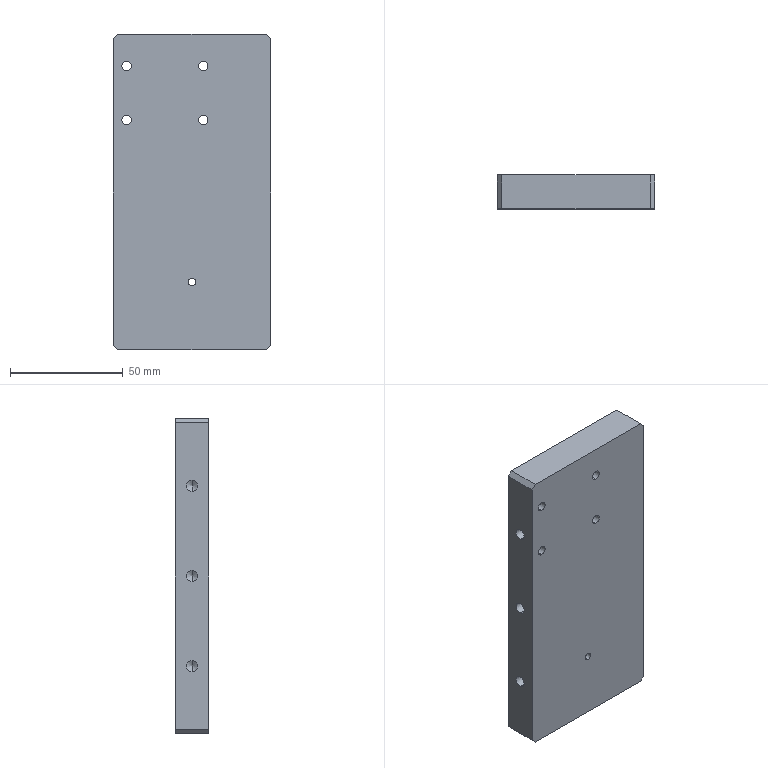Part | SolidWorks | features BaseBody 1 | 1 solid | 40 faces | box 70 x 15 x 140 mm | volume 144202 mm3 | cylinder 20 | cone 10 | plane 10 | commonest cylinder face diameters 5 x10 4.2 x8 3.3 x2
STEP:
#1=CARTESIAN_POINT('',(40.,15.,-40.1));
#2=VERTEX_POINT('',#1);
#3=CARTESIAN_POINT('',(40.,15.,-35.9));
#4=VERTEX_POINT('',#3);
#5=CARTESIAN_POINT('',(40.,15.,-38.));
#6=DIRECTION('',(0.,1.,0.));
#7=DIRECTION('',(0.,0.,-1.));
#8=AXIS2_PLACEMENT_3D('',#5,#6,#7);
#9=CIRCLE('',#8,2.1);
#10=EDGE_CURVE('',#2,#4,#9,.T.);
#11=ORIENTED_EDGE('',*,*,#10,.T.);
#12=CARTESIAN_POINT('',(40.,0.,-35.9));
#13=VERTEX_POINT('',#12);
#14=CARTESIAN_POINT('',(40.,0.,-35.9));
#15=DIRECTION('',(0.,-1.,0.));
#16=VECTOR('',#15,1000.);
#17=LINE('',#14,#16);
#18=EDGE_CURVE('',#4,#13,#17,.T.);
#19=ORIENTED_EDGE('',*,*,#18,.T.);
#20=CARTESIAN_POINT('',(40.,0.,-40.1));
#21=VERTEX_POINT('',#20);
#22=CARTESIAN_POINT('',(40.,0.,-38.));
#23=DIRECTION('',(0.,1.,0.));
#24=DIRECTION('',(0.,0.,-1.));
#25=AXIS2_PLACEMENT_3D('',#22,#23,#24);
#26=CIRCLE('',#25,2.1);
#27=EDGE_CURVE('',#21,#13,#26,.T.);
#28=ORIENTED_EDGE('',*,*,#27,.F.);
#29=CARTESIAN_POINT('',(40.,0.,-40.1));
#30=DIRECTION('',(0.,-1.,0.));
#31=VECTOR('',#30,1000.);
#32=LINE('',#29,#31);
#33=EDGE_CURVE('',#2,#21,#32,.T.);
#34=ORIENTED_EDGE('',*,*,#33,.F.);
#35=EDGE_LOOP('',(#11,#19,#28,#34));
#36=FACE_OUTER_BOUND('',#35,.T.);
#37=CARTESIAN_POINT('',(40.,0.,-38.));
#38=DIRECTION('',(0.,-1.,0.));
#39=DIRECTION('',(0.,0.,-1.));
#40=AXIS2_PLACEMENT_3D('',#37,#38,#39);
#41=CYLINDRICAL_SURFACE('',#40,2.1);
#42=ADVANCED_FACE('',(#36),#41,.F.);
#43=CARTESIAN_POINT('',(40.,15.,-16.1));
#44=VERTEX_POINT('',#43);
#45=CARTESIAN_POINT('',(40.,15.,-11.9));
#46=VERTEX_POINT('',#45);
#47=CARTESIAN_POINT('',(40.,15.,-14.));
#48=DIRECTION('',(0.,1.,0.));
#49=DIRECTION('',(0.,0.,-1.));
#50=AXIS2_PLACEMENT_3D('',#47,#48,#49);
#51=CIRCLE('',#50,2.1);
#52=EDGE_CURVE('',#44,#46,#51,.T.);
#53=ORIENTED_EDGE('',*,*,#52,.T.);
#54=CARTESIAN_POINT('',(40.,0.,-11.9));
#55=VERTEX_POINT('',#54);
#56=CARTESIAN_POINT('',(40.,0.,-11.9));
#57=DIRECTION('',(0.,-1.,0.));
#58=VECTOR('',#57,1000.);
#59=LINE('',#56,#58);
#60=EDGE_CURVE('',#46,#55,#59,.T.);
#61=ORIENTED_EDGE('',*,*,#60,.T.);
#62=CARTESIAN_POINT('',(40.,0.,-16.1));
#63=VERTEX_POINT('',#62);
#64=CARTESIAN_POINT('',(40.,0.,-14.));
#65=DIRECTION('',(0.,1.,0.));
#66=DIRECTION('',(0.,0.,-1.));
#67=AXIS2_PLACEMENT_3D('',#64,#65,#66);
#68=CIRCLE('',#67,2.1);
#69=EDGE_CURVE('',#63,#55,#68,.T.);
#70=ORIENTED_EDGE('',*,*,#69,.F.);
#71=CARTESIAN_POINT('',(40.,0.,-16.1));
#72=DIRECTION('',(0.,-1.,0.));
#73=VECTOR('',#72,1000.);
#74=LINE('',#71,#73);
#75=EDGE_CURVE('',#44,#63,#74,.T.);
#76=ORIENTED_EDGE('',*,*,#75,.F.);
#77=EDGE_LOOP('',(#53,#61,#70,#76));
#78=FACE_OUTER_BOUND('',#77,.T.);
#79=CARTESIAN_POINT('',(40.,0.,-14.));
#80=DIRECTION('',(0.,-1.,0.));
#81=DIRECTION('',(0.,0.,-1.));
#82=AXIS2_PLACEMENT_3D('',#79,#80,#81);
#83=CYLINDRICAL_SURFACE('',#82,2.1);
#84=ADVANCED_FACE('',(#78),#83,.F.);
#85=CARTESIAN_POINT('',(6.,15.,-16.1));
#86=VERTEX_POINT('',#85);
#87=CARTESIAN_POINT('',(6.,15.,-11.9));
#88=VERTEX_POINT('',#87);
#89=CARTESIAN_POINT('',(6.,15.,-14.));
#90=DIRECTION('',(0.,1.,0.));
#91=DIRECTION('',(0.,0.,-1.));
#92=AXIS2_PLACEMENT_3D('',#89,#90,#91);
#93=CIRCLE('',#92,2.1);
#94=EDGE_CURVE('',#86,#88,#93,.T.);
#95=ORIENTED_EDGE('',*,*,#94,.T.);
#96=CARTESIAN_POINT('',(6.,0.,-11.9));
#97=VERTEX_POINT('',#96);
#98=CARTESIAN_POINT('',(6.,0.,-11.9));
#99=DIRECTION('',(0.,-1.,0.));
#100=VECTOR('',#99,1000.);
#101=LINE('',#98,#100);
#102=EDGE_CURVE('',#88,#97,#101,.T.);
#103=ORIENTED_EDGE('',*,*,#102,.T.);
#104=CARTESIAN_POINT('',(6.,0.,-16.1));
#105=VERTEX_POINT('',#104);
#106=CARTESIAN_POINT('',(6.,0.,-14.));
#107=DIRECTION('',(0.,1.,0.));
#108=DIRECTION('',(0.,0.,-1.));
#109=AXIS2_PLACEMENT_3D('',#106,#107,#108);
#110=CIRCLE('',#109,2.1);
#111=EDGE_CURVE('',#105,#97,#110,.T.);
#112=ORIENTED_EDGE('',*,*,#111,.F.);
#113=CARTESIAN_POINT('',(6.,0.,-16.1));
#114=DIRECTION('',(0.,-1.,0.));
#115=VECTOR('',#114,1000.);
#116=LINE('',#113,#115);
#117=EDGE_CURVE('',#86,#105,#116,.T.);
#118=ORIENTED_EDGE('',*,*,#117,.F.);
#119=EDGE_LOOP('',(#95,#103,#112,#118));
#120=FACE_OUTER_BOUND('',#119,.T.);
#121=CARTESIAN_POINT('',(6.,0.,-14.));
#122=DIRECTION('',(0.,-1.,0.));
#123=DIRECTION('',(0.,0.,-1.));
#124=AXIS2_PLACEMENT_3D('',#121,#122,#123);
#125=CYLINDRICAL_SURFACE('',#124,2.1);
#126=ADVANCED_FACE('',(#120),#125,.F.);
#127=CARTESIAN_POINT('',(6.,15.,-40.1));
#128=VERTEX_POINT('',#127);
#129=CARTESIAN_POINT('',(6.,15.,-35.9));
#130=VERTEX_POINT('',#129);
#131=CARTESIAN_POINT('',(6.,15.,-38.));
#132=DIRECTION('',(0.,1.,0.));
#133=DIRECTION('',(0.,0.,-1.));
#134=AXIS2_PLACEMENT_3D('',#131,#132,#133);
#135=CIRCLE('',#134,2.1);
#136=EDGE_CURVE('',#128,#130,#135,.T.);
#137=ORIENTED_EDGE('',*,*,#136,.T.);
#138=CARTESIAN_POINT('',(6.,0.,-35.9));
#139=VERTEX_POINT('',#138);
#140=CARTESIAN_POINT('',(6.,0.,-35.9));
#141=DIRECTION('',(0.,-1.,0.));
#142=VECTOR('',#141,1000.);
#143=LINE('',#140,#142);
#144=EDGE_CURVE('',#130,#139,#143,.T.);
#145=ORIENTED_EDGE('',*,*,#144,.T.);
#146=CARTESIAN_POINT('',(6.,0.,-40.1));
#147=VERTEX_POINT('',#146);
#148=CARTESIAN_POINT('',(6.,0.,-38.));
#149=DIRECTION('',(0.,1.,0.));
#150=DIRECTION('',(0.,0.,-1.));
#151=AXIS2_PLACEMENT_3D('',#148,#149,#150);
#152=CIRCLE('',#151,2.1);
#153=EDGE_CURVE('',#147,#139,#152,.T.);
#154=ORIENTED_EDGE('',*,*,#153,.F.);
#155=CARTESIAN_POINT('',(6.,0.,-40.1));
#156=DIRECTION('',(0.,-1.,0.));
#157=VECTOR('',#156,1000.);
#158=LINE('',#155,#157);
#159=EDGE_CURVE('',#128,#147,#158,.T.);
#160=ORIENTED_EDGE('',*,*,#159,.F.);
#161=EDGE_LOOP('',(#137,#145,#154,#160));
#162=FACE_OUTER_BOUND('',#161,.T.);
#163=CARTESIAN_POINT('',(6.,0.,-38.));
#164=DIRECTION('',(0.,-1.,0.));
#165=DIRECTION('',(0.,0.,-1.));
#166=AXIS2_PLACEMENT_3D('',#163,#164,#165);
#167=CYLINDRICAL_SURFACE('',#166,2.1);
#168=ADVANCED_FACE('',(#162),#167,.F.);
#169=CARTESIAN_POINT('',(35.,0.,-111.65));
#170=VERTEX_POINT('',#169);
#171=CARTESIAN_POINT('',(35.,0.,-108.35));
#172=VERTEX_POINT('',#171);
#173=CARTESIAN_POINT('',(35.,0.,-110.));
#174=DIRECTION('',(0.,1.,0.));
#175=DIRECTION('',(0.,0.,1.));
#176=AXIS2_PLACEMENT_3D('',#173,#174,#175);
#177=CIRCLE('',#176,1.65);
#178=EDGE_CURVE('',#170,#172,#177,.T.);
#179=ORIENTED_EDGE('',*,*,#178,.F.);
#180=CARTESIAN_POINT('',(35.,15.,-111.65));
#181=VERTEX_POINT('',#180);
#182=CARTESIAN_POINT('',(35.,15.,-111.65));
#183=DIRECTION('',(0.,1.,0.));
#184=VECTOR('',#183,1000.);
#185=LINE('',#182,#184);
#186=EDGE_CURVE('',#170,#181,#185,.T.);
#187=ORIENTED_EDGE('',*,*,#186,.T.);
#188=CARTESIAN_POINT('',(35.,15.,-108.35));
#189=VERTEX_POINT('',#188);
#190=CARTESIAN_POINT('',(35.,15.,-110.));
#191=DIRECTION('',(0.,1.,0.));
#192=DIRECTION('',(0.,0.,1.));
#193=AXIS2_PLACEMENT_3D('',#190,#191,#192);
#194=CIRCLE('',#193,1.65);
#195=EDGE_CURVE('',#181,#189,#194,.T.);
#196=ORIENTED_EDGE('',*,*,#195,.T.);
#197=CARTESIAN_POINT('',(35.,15.,-108.35));
#198=DIRECTION('',(0.,1.,0.));
#199=VECTOR('',#198,1000.);
#200=LINE('',#197,#199);
#201=EDGE_CURVE('',#172,#189,#200,.T.);
#202=ORIENTED_EDGE('',*,*,#201,.F.);
#203=EDGE_LOOP('',(#179,#187,#196,#202));
#204=FACE_OUTER_BOUND('',#203,.T.);
#205=CARTESIAN_POINT('',(35.,15.,-110.));
#206=DIRECTION('',(0.,1.,0.));
#207=DIRECTION('',(0.,0.,1.));
#208=AXIS2_PLACEMENT_3D('',#205,#206,#207);
#209=CYLINDRICAL_SURFACE('',#208,1.65);
#210=ADVANCED_FACE('',(#204),#209,.F.);
#211=CARTESIAN_POINT('',(17.,7.5,-32.5));
#212=VERTEX_POINT('',#211);
#213=CARTESIAN_POINT('',(17.,7.5,-27.5));
#214=VERTEX_POINT('',#213);
#215=CARTESIAN_POINT('',(17.,7.5,-30.));
#216=DIRECTION('',(-1.,0.,0.));
#217=DIRECTION('',(0.,0.,1.));
#218=AXIS2_PLACEMENT_3D('',#215,#216,#217);
#219=CIRCLE('',#218,2.5);
#220=EDGE_CURVE('',#212,#214,#219,.T.);
#221=ORIENTED_EDGE('',*,*,#220,.F.);
#222=CARTESIAN_POINT('',(0.,7.5,-32.5));
#223=VERTEX_POINT('',#222);
#224=CARTESIAN_POINT('',(0.,7.5,-32.5));
#225=DIRECTION('',(-1.,0.,0.));
#226=VECTOR('',#225,1000.);
#227=LINE('',#224,#226);
#228=EDGE_CURVE('',#212,#223,#227,.T.);
#229=ORIENTED_EDGE('',*,*,#228,.T.);
#230=CARTESIAN_POINT('',(0.,7.5,-27.5));
#231=VERTEX_POINT('',#230);
#232=CARTESIAN_POINT('',(0.,7.5,-30.));
#233=DIRECTION('',(-1.,0.,0.));
#234=DIRECTION('',(0.,0.,1.));
#235=AXIS2_PLACEMENT_3D('',#232,#233,#234);
#236=CIRCLE('',#235,2.5);
#237=EDGE_CURVE('',#223,#231,#236,.T.);
#238=ORIENTED_EDGE('',*,*,#237,.T.);
#239=CARTESIAN_POINT('',(0.,7.5,-27.5));
#240=DIRECTION('',(-1.,0.,0.));
#241=VECTOR('',#240,1000.);
#242=LINE('',#239,#241);
#243=EDGE_CURVE('',#214,#231,#242,.T.);
#244=ORIENTED_EDGE('',*,*,#243,.F.);
#245=EDGE_LOOP('',(#221,#229,#238,#244));
#246=FACE_OUTER_BOUND('',#245,.T.);
#247=CARTESIAN_POINT('',(0.,7.5,-30.));
#248=DIRECTION('',(-1.,0.,0.));
#249=DIRECTION('',(0.,0.,1.));
#250=AXIS2_PLACEMENT_3D('',#247,#248,#249);
#251=CYLINDRICAL_SURFACE('',#250,2.5);
#252=ADVANCED_FACE('',(#246),#251,.F.);
#253=CARTESIAN_POINT('',(17.,7.5,-112.5));
#254=VERTEX_POINT('',#253);
#255=CARTESIAN_POINT('',(17.,7.5,-107.5));
#256=VERTEX_POINT('',#255);
#257=CARTESIAN_POINT('',(17.,7.5,-110.));
#258=DIRECTION('',(-1.,0.,0.));
#259=DIRECTION('',(0.,0.,1.));
#260=AXIS2_PLACEMENT_3D('',#257,#258,#259);
#261=CIRCLE('',#260,2.5);
#262=EDGE_CURVE('',#254,#256,#261,.T.);
#263=ORIENTED_EDGE('',*,*,#262,.F.);
#264=CARTESIAN_POINT('',(0.,7.5,-112.5));
#265=VERTEX_POINT('',#264);
#266=CARTESIAN_POINT('',(0.,7.5,-112.5));
#267=DIRECTION('',(-1.,0.,0.));
#268=VECTOR('',#267,1000.);
#269=LINE('',#266,#268);
#270=EDGE_CURVE('',#254,#265,#269,.T.);
#271=ORIENTED_EDGE('',*,*,#270,.T.);
#272=CARTESIAN_POINT('',(0.,7.5,-107.5));
#273=VERTEX_POINT('',#272);
#274=CARTESIAN_POINT('',(0.,7.5,-110.));
#275=DIRECTION('',(-1.,0.,0.));
#276=DIRECTION('',(0.,0.,1.));
#277=AXIS2_PLACEMENT_3D('',#274,#275,#276);
#278=CIRCLE('',#277,2.5);
#279=EDGE_CURVE('',#265,#273,#278,.T.);
#280=ORIENTED_EDGE('',*,*,#279,.T.);
#281=CARTESIAN_POINT('',(0.,7.5,-107.5));
#282=DIRECTION('',(-1.,0.,0.));
#283=VECTOR('',#282,1000.);
#284=LINE('',#281,#283);
#285=EDGE_CURVE('',#256,#273,#284,.T.);
#286=ORIENTED_EDGE('',*,*,#285,.F.);
#287=EDGE_LOOP('',(#263,#271,#280,#286));
#288=FACE_OUTER_BOUND('',#287,.T.);
#289=CARTESIAN_POINT('',(0.,7.5,-110.));
#290=DIRECTION('',(-1.,0.,0.));
#291=DIRECTION('',(0.,0.,1.));
#292=AXIS2_PLACEMENT_3D('',#289,#290,#291);
#293=CYLINDRICAL_SURFACE('',#292,2.5);
#294=ADVANCED_FACE('',(#288),#293,.F.);
#295=CARTESIAN_POINT('',(17.,7.5,-72.5));
#296=VERTEX_POINT('',#295);
#297=CARTESIAN_POINT('',(17.,7.5,-67.5));
#298=VERTEX_POINT('',#297);
#299=CARTESIAN_POINT('',(17.,7.5,-70.));
#300=DIRECTION('',(-1.,0.,0.));
#301=DIRECTION('',(0.,0.,1.));
#302=AXIS2_PLACEMENT_3D('',#299,#300,#301);
#303=CIRCLE('',#302,2.5);
#304=EDGE_CURVE('',#296,#298,#303,.T.);
#305=ORIENTED_EDGE('',*,*,#304,.F.);
#306=CARTESIAN_POINT('',(0.,7.5,-72.5));
#307=VERTEX_POINT('',#306);
#308=CARTESIAN_POINT('',(0.,7.5,-72.5));
#309=DIRECTION('',(-1.,0.,0.));
#310=VECTOR('',#309,1000.);
#311=LINE('',#308,#310);
#312=EDGE_CURVE('',#296,#307,#311,.T.);
#313=ORIENTED_EDGE('',*,*,#312,.T.);
#314=CARTESIAN_POINT('',(0.,7.5,-67.5));
#315=VERTEX_POINT('',#314);
#316=CARTESIAN_POINT('',(0.,7.5,-70.));
#317=DIRECTION('',(-1.,0.,0.));
#318=DIRECTION('',(0.,0.,1.));
#319=AXIS2_PLACEMENT_3D('',#316,#317,#318);
#320=CIRCLE('',#319,2.5);
#321=EDGE_CURVE('',#307,#315,#320,.T.);
#322=ORIENTED_EDGE('',*,*,#321,.T.);
#323=CARTESIAN_POINT('',(0.,7.5,-67.5));
#324=DIRECTION('',(-1.,0.,0.));
#325=VECTOR('',#324,1000.);
#326=LINE('',#323,#325);
#327=EDGE_CURVE('',#298,#315,#326,.T.);
#328=ORIENTED_EDGE('',*,*,#327,.F.);
#329=EDGE_LOOP('',(#305,#313,#322,#328));
#330=FACE_OUTER_BOUND('',#329,.T.);
#331=CARTESIAN_POINT('',(0.,7.5,-70.));
#332=DIRECTION('',(-1.,0.,0.));
#333=DIRECTION('',(0.,0.,1.));
#334=AXIS2_PLACEMENT_3D('',#331,#332,#333);
#335=CYLINDRICAL_SURFACE('',#334,2.5);
#336=ADVANCED_FACE('',(#330),#335,.F.);
#337=CARTESIAN_POINT('',(62.5,7.5,-123.));
#338=VERTEX_POINT('',#337);
#339=CARTESIAN_POINT('',(60.,5.,-123.));
#340=VERTEX_POINT('',#339);
#341=CARTESIAN_POINT('',(60.,7.5,-123.));
#342=DIRECTION('',(0.,0.,-1.));
#343=DIRECTION('',(-1.,0.,0.));
#344=AXIS2_PLACEMENT_3D('',#341,#342,#343);
#345=CIRCLE('',#344,2.5);
#346=EDGE_CURVE('',#338,#340,#345,.T.);
#347=ORIENTED_EDGE('',*,*,#346,.F.);
#348=CARTESIAN_POINT('',(62.5,7.5,-140.));
#349=VERTEX_POINT('',#348);
#350=CARTESIAN_POINT('',(62.5,7.5,-140.));
#351=DIRECTION('',(0.,0.,-1.));
#352=VECTOR('',#351,1000.);
#353=LINE('',#350,#352);
#354=EDGE_CURVE('',#338,#349,#353,.T.);
#355=ORIENTED_EDGE('',*,*,#354,.T.);
#356=CARTESIAN_POINT('',(57.5,7.5,-140.));
#357=VERTEX_POINT('',#356);
#358=CARTESIAN_POINT('',(60.,7.5,-140.));
#359=DIRECTION('',(0.,0.,-1.));
#360=DIRECTION('',(-1.,0.,0.));
#361=AXIS2_PLACEMENT_3D('',#358,#359,#360);
#362=CIRCLE('',#361,2.5);
#363=EDGE_CURVE('',#349,#357,#362,.T.);
#364=ORIENTED_EDGE('',*,*,#363,.T.);
#365=CARTESIAN_POINT('',(57.5,7.5,-123.));
#366=VERTEX_POINT('',#365);
#367=CARTESIAN_POINT('',(57.5,7.5,-140.));
#368=DIRECTION('',(0.,0.,-1.));
#369=VECTOR('',#368,1000.);
#370=LINE('',#367,#369);
#371=EDGE_CURVE('',#366,#357,#370,.T.);
#372=ORIENTED_EDGE('',*,*,#371,.F.);
#373=CARTESIAN_POINT('',(60.,7.5,-123.));
#374=DIRECTION('',(0.,0.,-1.));
#375=DIRECTION('',(-1.,0.,0.));
#376=AXIS2_PLACEMENT_3D('',#373,#374,#375);
#377=CIRCLE('',#376,2.5);
#378=EDGE_CURVE('',#340,#366,#377,.T.);
#379=ORIENTED_EDGE('',*,*,#378,.F.);
#380=EDGE_LOOP('',(#347,#355,#364,#372,#379));
#381=FACE_OUTER_BOUND('',#380,.T.);
#382=CARTESIAN_POINT('',(60.,7.5,-140.));
#383=DIRECTION('',(0.,0.,-1.));
#384=DIRECTION('',(-1.,0.,0.));
#385=AXIS2_PLACEMENT_3D('',#382,#383,#384);
#386=CYLINDRICAL_SURFACE('',#385,2.5);
#387=ADVANCED_FACE('',(#381),#386,.F.);
#388=CARTESIAN_POINT('',(22.5,7.5,-123.));
#389=VERTEX_POINT('',#388);
#390=CARTESIAN_POINT('',(20.,5.,-123.));
#391=VERTEX_POINT('',#390);
#392=CARTESIAN_POINT('',(20.,7.5,-123.));
#393=DIRECTION('',(0.,0.,-1.));
#394=DIRECTION('',(-1.,0.,0.));
#395=AXIS2_PLACEMENT_3D('',#392,#393,#394);
#396=CIRCLE('',#395,2.5);
#397=EDGE_CURVE('',#389,#391,#396,.T.);
#398=ORIENTED_EDGE('',*,*,#397,.F.);
#399=CARTESIAN_POINT('',(22.5,7.5,-140.));
#400=VERTEX_POINT('',#399);
#401=CARTESIAN_POINT('',(22.5,7.5,-140.));
#402=DIRECTION('',(0.,0.,-1.));
#403=VECTOR('',#402,1000.);
#404=LINE('',#401,#403);
#405=EDGE_CURVE('',#389,#400,#404,.T.);
#406=ORIENTED_EDGE('',*,*,#405,.T.);
#407=CARTESIAN_POINT('',(17.5,7.5,-140.));
#408=VERTEX_POINT('',#407);
#409=CARTESIAN_POINT('',(20.,7.5,-140.));
#410=DIRECTION('',(0.,0.,-1.));
#411=DIRECTION('',(-1.,0.,0.));
#412=AXIS2_PLACEMENT_3D('',#409,#410,#411);
#413=CIRCLE('',#412,2.5);
#414=EDGE_CURVE('',#400,#408,#413,.T.);
#415=ORIENTED_EDGE('',*,*,#414,.T.);
#416=CARTESIAN_POINT('',(17.5,7.5,-123.));
#417=VERTEX_POINT('',#416);
#418=CARTESIAN_POINT('',(17.5,7.5,-140.));
#419=DIRECTION('',(0.,0.,-1.));
#420=VECTOR('',#419,1000.);
#421=LINE('',#418,#420);
#422=EDGE_CURVE('',#417,#408,#421,.T.);
#423=ORIENTED_EDGE('',*,*,#422,.F.);
#424=CARTESIAN_POINT('',(20.,7.5,-123.));
#425=DIRECTION('',(0.,0.,-1.));
#426=DIRECTION('',(-1.,0.,0.));
#427=AXIS2_PLACEMENT_3D('',#424,#425,#426);
#428=CIRCLE('',#427,2.5);
#429=EDGE_CURVE('',#391,#417,#428,.T.);
#430=ORIENTED_EDGE('',*,*,#429,.F.);
#431=EDGE_LOOP('',(#398,#406,#415,#423,#430));
#432=FACE_OUTER_BOUND('',#431,.T.);
#433=CARTESIAN_POINT('',(20.,7.5,-140.));
#434=DIRECTION('',(0.,0.,-1.));
#435=DIRECTION('',(-1.,0.,0.));
#436=AXIS2_PLACEMENT_3D('',#433,#434,#435);
#437=CYLINDRICAL_SURFACE('',#436,2.5);
#438=ADVANCED_FACE('',(#432),#437,.F.);
#439=CARTESIAN_POINT('',(18.502,7.5,-30.));
#440=VERTEX_POINT('',#439);
#441=CARTESIAN_POINT('',(17.,7.5,-27.5));
#442=DIRECTION('',(-0.515,0.,0.8572));
#443=VECTOR('',#442,1000.);
#444=LINE('',#441,#443);
#445=EDGE_CURVE('',#440,#214,#444,.T.);
#446=ORIENTED_EDGE('',*,*,#445,.F.);
#447=CARTESIAN_POINT('',(17.,7.5,-32.5));
#448=DIRECTION('',(-0.515,0.,-0.8572));
#449=VECTOR('',#448,1000.);
#450=LINE('',#447,#449);
#451=EDGE_CURVE('',#440,#212,#450,.T.);
#452=ORIENTED_EDGE('',*,*,#451,.T.);
#453=ORIENTED_EDGE('',*,*,#220,.T.);
#454=EDGE_LOOP('',(#446,#452,#453));
#455=FACE_OUTER_BOUND('',#454,.T.);
#456=CARTESIAN_POINT('',(17.,7.5,-30.));
#457=DIRECTION('',(-1.,0.,0.));
#458=DIRECTION('',(0.,0.,1.));
#459=AXIS2_PLACEMENT_3D('',#456,#457,#458);
#460=CONICAL_SURFACE('',#459,2.5,1.03);
#461=ADVANCED_FACE('',(#455),#460,.F.);
#462=CARTESIAN_POINT('',(18.502,7.5,-110.));
#463=VERTEX_POINT('',#462);
#464=CARTESIAN_POINT('',(17.,7.5,-107.5));
#465=DIRECTION('',(-0.515,0.,0.8572));
#466=VECTOR('',#465,1000.);
#467=LINE('',#464,#466);
#468=EDGE_CURVE('',#463,#256,#467,.T.);
#469=ORIENTED_EDGE('',*,*,#468,.F.);
#470=CARTESIAN_POINT('',(17.,7.5,-112.5));
#471=DIRECTION('',(-0.515,0.,-0.8572));
#472=VECTOR('',#471,1000.);
#473=LINE('',#470,#472);
#474=EDGE_CURVE('',#463,#254,#473,.T.);
#475=ORIENTED_EDGE('',*,*,#474,.T.);
#476=ORIENTED_EDGE('',*,*,#262,.T.);
#477=EDGE_LOOP('',(#469,#475,#476));
#478=FACE_OUTER_BOUND('',#477,.T.);
#479=CARTESIAN_POINT('',(17.,7.5,-110.));
#480=DIRECTION('',(-1.,0.,0.));
#481=DIRECTION('',(0.,0.,1.));
#482=AXIS2_PLACEMENT_3D('',#479,#480,#481);
#483=CONICAL_SURFACE('',#482,2.5,1.03);
#484=ADVANCED_FACE('',(#478),#483,.F.);
#485=CARTESIAN_POINT('',(18.502,7.5,-70.));
#486=VERTEX_POINT('',#485);
#487=CARTESIAN_POINT('',(17.,7.5,-67.5));
#488=DIRECTION('',(-0.515,0.,0.8572));
#489=VECTOR('',#488,1000.);
#490=LINE('',#487,#489);
#491=EDGE_CURVE('',#486,#298,#490,.T.);
#492=ORIENTED_EDGE('',*,*,#491,.F.);
#493=CARTESIAN_POINT('',(17.,7.5,-72.5));
#494=DIRECTION('',(-0.515,0.,-0.8572));
#495=VECTOR('',#494,1000.);
#496=LINE('',#493,#495);
#497=EDGE_CURVE('',#486,#296,#496,.T.);
#498=ORIENTED_EDGE('',*,*,#497,.T.);
#499=ORIENTED_EDGE('',*,*,#304,.T.);
#500=EDGE_LOOP('',(#492,#498,#499));
#501=FACE_OUTER_BOUND('',#500,.T.);
#502=CARTESIAN_POINT('',(17.,7.5,-70.));
#503=DIRECTION('',(-1.,0.,0.));
#504=DIRECTION('',(0.,0.,1.));
#505=AXIS2_PLACEMENT_3D('',#502,#503,#504);
#506=CONICAL_SURFACE('',#505,2.5,1.03);
#507=ADVANCED_FACE('',(#501),#506,.F.);
#508=CARTESIAN_POINT('',(60.,7.5,-121.498));
#509=VERTEX_POINT('',#508);
#510=CARTESIAN_POINT('',(60.,10.,-123.));
#511=VERTEX_POINT('',#510);
#512=CARTESIAN_POINT('',(60.,10.,-123.));
#513=DIRECTION('',(0.,0.8572,-0.515));
#514=VECTOR('',#513,1000.);
#515=LINE('',#512,#514);
#516=EDGE_CURVE('',#509,#511,#515,.T.);
#517=ORIENTED_EDGE('',*,*,#516,.F.);
#518=CARTESIAN_POINT('',(60.,5.,-123.));
#519=DIRECTION('',(0.,-0.8572,-0.515));
#520=VECTOR('',#519,1000.);
#521=LINE('',#518,#520);
#522=EDGE_CURVE('',#509,#340,#521,.T.);
#523=ORIENTED_EDGE('',*,*,#522,.T.);
#524=ORIENTED_EDGE('',*,*,#378,.T.);
#525=CARTESIAN_POINT('',(60.,7.5,-123.));
#526=DIRECTION('',(0.,0.,-1.));
#527=DIRECTION('',(-1.,0.,0.));
#528=AXIS2_PLACEMENT_3D('',#525,#526,#527);
#529=CIRCLE('',#528,2.5);
#530=EDGE_CURVE('',#366,#511,#529,.T.);
#531=ORIENTED_EDGE('',*,*,#530,.T.);
#532=EDGE_LOOP('',(#517,#523,#524,#531));
#533=FACE_OUTER_BOUND('',#532,.T.);
#534=CARTESIAN_POINT('',(60.,7.5,-123.));
#535=DIRECTION('',(0.,0.,-1.));
#536=DIRECTION('',(0.,1.,0.));
#537=AXIS2_PLACEMENT_3D('',#534,#535,#536);
#538=CONICAL_SURFACE('',#537,2.5,1.03);
#539=ADVANCED_FACE('',(#533),#538,.F.);
#540=CARTESIAN_POINT('',(20.,7.5,-121.498));
#541=VERTEX_POINT('',#540);
#542=CARTESIAN_POINT('',(20.,10.,-123.));
#543=VERTEX_POINT('',#542);
#544=CARTESIAN_POINT('',(20.,10.,-123.));
#545=DIRECTION('',(0.,0.8572,-0.515));
#546=VECTOR('',#545,1000.);
#547=LINE('',#544,#546);
#548=EDGE_CURVE('',#541,#543,#547,.T.);
#549=ORIENTED_EDGE('',*,*,#548,.F.);
#550=CARTESIAN_POINT('',(20.,5.,-123.));
#551=DIRECTION('',(0.,-0.8572,-0.515));
#552=VECTOR('',#551,1000.);
#553=LINE('',#550,#552);
#554=EDGE_CURVE('',#541,#391,#553,.T.);
#555=ORIENTED_EDGE('',*,*,#554,.T.);
#556=ORIENTED_EDGE('',*,*,#429,.T.);
#557=CARTESIAN_POINT('',(20.,7.5,-123.));
#558=DIRECTION('',(0.,0.,-1.));
#559=DIRECTION('',(-1.,0.,0.));
#560=AXIS2_PLACEMENT_3D('',#557,#558,#559);
#561=CIRCLE('',#560,2.5);
#562=EDGE_CURVE('',#417,#543,#561,.T.);
#563=ORIENTED_EDGE('',*,*,#562,.T.);
#564=EDGE_LOOP('',(#549,#555,#556,#563));
#565=FACE_OUTER_BOUND('',#564,.T.);
#566=CARTESIAN_POINT('',(20.,7.5,-123.));
#567=DIRECTION('',(0.,0.,-1.));
#568=DIRECTION('',(0.,1.,0.));
#569=AXIS2_PLACEMENT_3D('',#566,#567,#568);
#570=CONICAL_SURFACE('',#569,2.5,1.03);
#571=ADVANCED_FACE('',(#565),#570,.F.);
#572=CARTESIAN_POINT('',(2.,15.,0.));
#573=VERTEX_POINT('',#572);
#574=CARTESIAN_POINT('',(0.,15.,-2.));
#575=VERTEX_POINT('',#574);
#576=CARTESIAN_POINT('',(2.,15.,0.));
#577=DIRECTION('',(-0.7071,0.,-0.7071));
#578=VECTOR('',#577,1000.);
#579=LINE('',#576,#578);
#580=EDGE_CURVE('',#573,#575,#579,.T.);
#581=ORIENTED_EDGE('',*,*,#580,.F.);
#582=CARTESIAN_POINT('',(68.,15.,0.));
#583=VERTEX_POINT('',#582);
#584=CARTESIAN_POINT('',(0.,15.,0.));
#585=DIRECTION('',(-1.,0.,0.));
#586=VECTOR('',#585,1000.);
#587=LINE('',#584,#586);
#588=EDGE_CURVE('',#583,#573,#587,.T.);
#589=ORIENTED_EDGE('',*,*,#588,.F.);
#590=CARTESIAN_POINT('',(70.,15.,-2.));
#591=VERTEX_POINT('',#590);
#592=CARTESIAN_POINT('',(70.,15.,-2.));
#593=DIRECTION('',(-0.7071,0.,0.7071));
#594=VECTOR('',#593,1000.);
#595=LINE('',#592,#594);
#596=EDGE_CURVE('',#591,#583,#595,.T.);
#597=ORIENTED_EDGE('',*,*,#596,.F.);
#598=CARTESIAN_POINT('',(70.,15.,-138.));
#599=VERTEX_POINT('',#598);
#600=CARTESIAN_POINT('',(70.,15.,0.));
#601=DIRECTION('',(0.,0.,1.));
#602=VECTOR('',#601,1000.);
#603=LINE('',#600,#602);
#604=EDGE_CURVE('',#599,#591,#603,.T.);
#605=ORIENTED_EDGE('',*,*,#604,.F.);
#606=CARTESIAN_POINT('',(68.,15.,-140.));
#607=VERTEX_POINT('',#606);
#608=CARTESIAN_POINT('',(68.,15.,-140.));
#609=DIRECTION('',(0.7071,0.,0.7071));
#610=VECTOR('',#609,1000.);
#611=LINE('',#608,#610);
#612=EDGE_CURVE('',#607,#599,#611,.T.);
#613=ORIENTED_EDGE('',*,*,#612,.F.);
#614=CARTESIAN_POINT('',(2.,15.,-140.));
#615=VERTEX_POINT('',#614);
#616=CARTESIAN_POINT('',(0.,15.,-140.));
#617=DIRECTION('',(1.,0.,0.));
#618=VECTOR('',#617,1000.);
#619=LINE('',#616,#618);
#620=EDGE_CURVE('',#615,#607,#619,.T.);
#621=ORIENTED_EDGE('',*,*,#620,.F.);
#622=CARTESIAN_POINT('',(0.,15.,-138.));
#623=VERTEX_POINT('',#622);
#624=CARTESIAN_POINT('',(0.,15.,-138.));
#625=DIRECTION('',(0.7071,0.,-0.7071));
#626=VECTOR('',#625,1000.);
#627=LINE('',#624,#626);
#628=EDGE_CURVE('',#623,#615,#627,.T.);
#629=ORIENTED_EDGE('',*,*,#628,.F.);
#630=CARTESIAN_POINT('',(0.,15.,0.));
#631=DIRECTION('',(0.,0.,-1.));
#632=VECTOR('',#631,1000.);
#633=LINE('',#630,#632);
#634=EDGE_CURVE('',#575,#623,#633,.T.);
#635=ORIENTED_EDGE('',*,*,#634,.F.);
#636=EDGE_LOOP('',(#581,#589,#597,#605,#613,#621,#629,#635));
#637=FACE_OUTER_BOUND('',#636,.T.);
#638=ORIENTED_EDGE('',*,*,#10,.F.);
#639=CARTESIAN_POINT('',(40.,15.,-38.));
#640=DIRECTION('',(0.,1.,0.));
#641=DIRECTION('',(0.,0.,-1.));
#642=AXIS2_PLACEMENT_3D('',#639,#640,#641);
#643=CIRCLE('',#642,2.1);
#644=EDGE_CURVE('',#4,#2,#643,.T.);
#645=ORIENTED_EDGE('',*,*,#644,.F.);
#646=EDGE_LOOP('',(#638,#645));
#647=FACE_BOUND('',#646,.T.);
#648=ORIENTED_EDGE('',*,*,#52,.F.);
#649=CARTESIAN_POINT('',(40.,15.,-14.));
#650=DIRECTION('',(0.,1.,0.));
#651=DIRECTION('',(0.,0.,-1.));
#652=AXIS2_PLACEMENT_3D('',#649,#650,#651);
#653=CIRCLE('',#652,2.1);
#654=EDGE_CURVE('',#46,#44,#653,.T.);
#655=ORIENTED_EDGE('',*,*,#654,.F.);
#656=EDGE_LOOP('',(#648,#655));
#657=FACE_BOUND('',#656,.T.);
#658=ORIENTED_EDGE('',*,*,#94,.F.);
#659=CARTESIAN_POINT('',(6.,15.,-14.));
#660=DIRECTION('',(0.,1.,0.));
#661=DIRECTION('',(0.,0.,-1.));
#662=AXIS2_PLACEMENT_3D('',#659,#660,#661);
#663=CIRCLE('',#662,2.1);
#664=EDGE_CURVE('',#88,#86,#663,.T.);
#665=ORIENTED_EDGE('',*,*,#664,.F.);
#666=EDGE_LOOP('',(#658,#665));
#667=FACE_BOUND('',#666,.T.);
#668=ORIENTED_EDGE('',*,*,#136,.F.);
#669=CARTESIAN_POINT('',(6.,15.,-38.));
#670=DIRECTION('',(0.,1.,0.));
#671=DIRECTION('',(0.,0.,-1.));
#672=AXIS2_PLACEMENT_3D('',#669,#670,#671);
#673=CIRCLE('',#672,2.1);
#674=EDGE_CURVE('',#130,#128,#673,.T.);
#675=ORIENTED_EDGE('',*,*,#674,.F.);
#676=EDGE_LOOP('',(#668,#675));
#677=FACE_BOUND('',#676,.T.);
#678=CARTESIAN_POINT('',(35.,15.,-110.));
#679=DIRECTION('',(0.,1.,0.));
#680=DIRECTION('',(0.,0.,1.));
#681=AXIS2_PLACEMENT_3D('',#678,#679,#680);
#682=CIRCLE('',#681,1.65);
#683=EDGE_CURVE('',#189,#181,#682,.T.);
#684=ORIENTED_EDGE('',*,*,#683,.F.);
#685=ORIENTED_EDGE('',*,*,#195,.F.);
#686=EDGE_LOOP('',(#684,#685));
#687=FACE_BOUND('',#686,.T.);
#688=CARTESIAN_POINT('',(0.,15.,0.));
#689=DIRECTION('',(0.,-1.,0.));
#690=DIRECTION('',(0.,0.,-1.));
#691=AXIS2_PLACEMENT_3D('',#688,#689,#690);
#692=PLANE('',#691);
#693=ADVANCED_FACE('',(#637,#647,#657,#667,#677,#687),#692,.F.);
#694=CARTESIAN_POINT('',(0.,0.,-2.));
#695=VERTEX_POINT('',#694);
#696=CARTESIAN_POINT('',(0.,15.,-2.));
#697=DIRECTION('',(0.,-1.,0.));
#698=VECTOR('',#697,1000.);
#699=LINE('',#696,#698);
#700=EDGE_CURVE('',#575,#695,#699,.T.);
#701=ORIENTED_EDGE('',*,*,#700,.F.);
#702=ORIENTED_EDGE('',*,*,#634,.T.);
#703=CARTESIAN_POINT('',(0.,0.,-138.));
#704=VERTEX_POINT('',#703);
#705=CARTESIAN_POINT('',(0.,15.,-138.));
#706=DIRECTION('',(0.,1.,0.));
#707=VECTOR('',#706,1000.);
#708=LINE('',#705,#707);
#709=EDGE_CURVE('',#704,#623,#708,.T.);
#710=ORIENTED_EDGE('',*,*,#709,.F.);
#711=CARTESIAN_POINT('',(0.,0.,0.));
#712=DIRECTION('',(0.,0.,-1.));
#713=VECTOR('',#712,1000.);
#714=LINE('',#711,#713);
#715=EDGE_CURVE('',#695,#704,#714,.T.);
#716=ORIENTED_EDGE('',*,*,#715,.F.);
#717=EDGE_LOOP('',(#701,#702,#710,#716));
#718=FACE_OUTER_BOUND('',#717,.T.);
#719=CARTESIAN_POINT('',(0.,7.5,-30.));
#720=DIRECTION('',(-1.,0.,0.));
#721=DIRECTION('',(0.,0.,1.));
#722=AXIS2_PLACEMENT_3D('',#719,#720,#721);
#723=CIRCLE('',#722,2.5);
#724=EDGE_CURVE('',#231,#223,#723,.T.);
#725=ORIENTED_EDGE('',*,*,#724,.F.);
#726=ORIENTED_EDGE('',*,*,#237,.F.);
#727=EDGE_LOOP('',(#725,#726));
#728=FACE_BOUND('',#727,.T.);
#729=CARTESIAN_POINT('',(0.,7.5,-110.));
#730=DIRECTION('',(-1.,0.,0.));
#731=DIRECTION('',(0.,0.,1.));
#732=AXIS2_PLACEMENT_3D('',#729,#730,#731);
#733=CIRCLE('',#732,2.5);
#734=EDGE_CURVE('',#273,#265,#733,.T.);
#735=ORIENTED_EDGE('',*,*,#734,.F.);
#736=ORIENTED_EDGE('',*,*,#279,.F.);
#737=EDGE_LOOP('',(#735,#736));
#738=FACE_BOUND('',#737,.T.);
#739=CARTESIAN_POINT('',(0.,7.5,-70.));
#740=DIRECTION('',(-1.,0.,0.));
#741=DIRECTION('',(0.,0.,1.));
#742=AXIS2_PLACEMENT_3D('',#739,#740,#741);
#743=CIRCLE('',#742,2.5);
#744=EDGE_CURVE('',#315,#307,#743,.T.);
#745=ORIENTED_EDGE('',*,*,#744,.F.);
#746=ORIENTED_EDGE('',*,*,#321,.F.);
#747=EDGE_LOOP('',(#745,#746));
#748=FACE_BOUND('',#747,.T.);
#749=CARTESIAN_POINT('',(0.,15.,0.));
#750=DIRECTION('',(1.,0.,0.));
#751=DIRECTION('',(0.,0.,-1.));
#752=AXIS2_PLACEMENT_3D('',#749,#750,#751);
#753=PLANE('',#752);
#754=ADVANCED_FACE('',(#718,#728,#738,#748),#753,.F.);
#755=ORIENTED_EDGE('',*,*,#700,.T.);
#756=CARTESIAN_POINT('',(2.,0.,0.));
#757=VERTEX_POINT('',#756);
#758=CARTESIAN_POINT('',(2.,0.,0.));
#759=DIRECTION('',(-0.7071,0.,-0.7071));
#760=VECTOR('',#759,1000.);
#761=LINE('',#758,#760);
#762=EDGE_CURVE('',#757,#695,#761,.T.);
#763=ORIENTED_EDGE('',*,*,#762,.F.);
#764=CARTESIAN_POINT('',(2.,15.,0.));
#765=DIRECTION('',(0.,-1.,0.));
#766=VECTOR('',#765,1000.);
#767=LINE('',#764,#766);
#768=EDGE_CURVE('',#573,#757,#767,.T.);
#769=ORIENTED_EDGE('',*,*,#768,.F.);
#770=ORIENTED_EDGE('',*,*,#580,.T.);
#771=EDGE_LOOP('',(#755,#763,#769,#770));
#772=FACE_OUTER_BOUND('',#771,.T.);
#773=CARTESIAN_POINT('',(2.,15.,0.));
#774=DIRECTION('',(0.7071,0.,-0.7071));
#775=DIRECTION('',(-0.7071,0.,-0.7071));
#776=AXIS2_PLACEMENT_3D('',#773,#774,#775);
#777=PLANE('',#776);
#778=ADVANCED_FACE('',(#772),#777,.F.);
#779=ORIENTED_EDGE('',*,*,#768,.T.);
#780=CARTESIAN_POINT('',(68.,0.,0.));
#781=VERTEX_POINT('',#780);
#782=CARTESIAN_POINT('',(0.,0.,0.));
#783=DIRECTION('',(-1.,0.,0.));
#784=VECTOR('',#783,1000.);
#785=LINE('',#782,#784);
#786=EDGE_CURVE('',#781,#757,#785,.T.);
#787=ORIENTED_EDGE('',*,*,#786,.F.);
#788=CARTESIAN_POINT('',(68.,15.,0.));
#789=DIRECTION('',(0.,-1.,0.));
#790=VECTOR('',#789,1000.);
#791=LINE('',#788,#790);
#792=EDGE_CURVE('',#583,#781,#791,.T.);
#793=ORIENTED_EDGE('',*,*,#792,.F.);
#794=ORIENTED_EDGE('',*,*,#588,.T.);
#795=EDGE_LOOP('',(#779,#787,#793,#794));
#796=FACE_OUTER_BOUND('',#795,.T.);
#797=CARTESIAN_POINT('',(0.,15.,0.));
#798=DIRECTION('',(0.,0.,-1.));
#799=DIRECTION('',(-1.,0.,0.));
#800=AXIS2_PLACEMENT_3D('',#797,#798,#799);
#801=PLANE('',#800);
#802=ADVANCED_FACE('',(#796),#801,.F.);
#803=ORIENTED_EDGE('',*,*,#792,.T.);
#804=CARTESIAN_POINT('',(70.,0.,-2.));
#805=VERTEX_POINT('',#804);
#806=CARTESIAN_POINT('',(70.,0.,-2.));
#807=DIRECTION('',(-0.7071,0.,0.7071));
#808=VECTOR('',#807,1000.);
#809=LINE('',#806,#808);
#810=EDGE_CURVE('',#805,#781,#809,.T.);
#811=ORIENTED_EDGE('',*,*,#810,.F.);
#812=CARTESIAN_POINT('',(70.,15.,-2.));
#813=DIRECTION('',(0.,-1.,0.));
#814=VECTOR('',#813,1000.);
#815=LINE('',#812,#814);
#816=EDGE_CURVE('',#591,#805,#815,.T.);
#817=ORIENTED_EDGE('',*,*,#816,.F.);
#818=ORIENTED_EDGE('',*,*,#596,.T.);
#819=EDGE_LOOP('',(#803,#811,#817,#818));
#820=FACE_OUTER_BOUND('',#819,.T.);
#821=CARTESIAN_POINT('',(70.,15.,-2.));
#822=DIRECTION('',(-0.7071,0.,-0.7071));
#823=DIRECTION('',(-0.7071,0.,0.7071));
#824=AXIS2_PLACEMENT_3D('',#821,#822,#823);
#825=PLANE('',#824);
#826=ADVANCED_FACE('',(#820),#825,.F.);
#827=CARTESIAN_POINT('',(70.,0.,-138.));
#828=VERTEX_POINT('',#827);
#829=CARTESIAN_POINT('',(70.,15.,-138.));
#830=DIRECTION('',(0.,-1.,0.));
#831=VECTOR('',#830,1000.);
#832=LINE('',#829,#831);
#833=EDGE_CURVE('',#599,#828,#832,.T.);
#834=ORIENTED_EDGE('',*,*,#833,.F.);
#835=ORIENTED_EDGE('',*,*,#604,.T.);
#836=ORIENTED_EDGE('',*,*,#816,.T.);
#837=CARTESIAN_POINT('',(70.,0.,0.));
#838=DIRECTION('',(0.,0.,1.));
#839=VECTOR('',#838,1000.);
#840=LINE('',#837,#839);
#841=EDGE_CURVE('',#828,#805,#840,.T.);
#842=ORIENTED_EDGE('',*,*,#841,.F.);
#843=EDGE_LOOP('',(#834,#835,#836,#842));
#844=FACE_OUTER_BOUND('',#843,.T.);
#845=CARTESIAN_POINT('',(70.,15.,0.));
#846=DIRECTION('',(-1.,0.,0.));
#847=DIRECTION('',(0.,0.,1.));
#848=AXIS2_PLACEMENT_3D('',#845,#846,#847);
#849=PLANE('',#848);
#850=ADVANCED_FACE('',(#844),#849,.F.);
#851=ORIENTED_EDGE('',*,*,#833,.T.);
#852=CARTESIAN_POINT('',(68.,0.,-140.));
#853=VERTEX_POINT('',#852);
#854=CARTESIAN_POINT('',(68.,0.,-140.));
#855=DIRECTION('',(0.7071,0.,0.7071));
#856=VECTOR('',#855,1000.);
#857=LINE('',#854,#856);
#858=EDGE_CURVE('',#853,#828,#857,.T.);
#859=ORIENTED_EDGE('',*,*,#858,.F.);
#860=CARTESIAN_POINT('',(68.,15.,-140.));
#861=DIRECTION('',(0.,-1.,0.));
#862=VECTOR('',#861,1000.);
#863=LINE('',#860,#862);
#864=EDGE_CURVE('',#607,#853,#863,.T.);
#865=ORIENTED_EDGE('',*,*,#864,.F.);
#866=ORIENTED_EDGE('',*,*,#612,.T.);
#867=EDGE_LOOP('',(#851,#859,#865,#866));
#868=FACE_OUTER_BOUND('',#867,.T.);
#869=CARTESIAN_POINT('',(68.,15.,-140.));
#870=DIRECTION('',(-0.7071,0.,0.7071));
#871=DIRECTION('',(0.7071,0.,0.7071));
#872=AXIS2_PLACEMENT_3D('',#869,#870,#871);
#873=PLANE('',#872);
#874=ADVANCED_FACE('',(#868),#873,.F.);
#875=CARTESIAN_POINT('',(2.,0.,-140.));
#876=VERTEX_POINT('',#875);
#877=CARTESIAN_POINT('',(2.,15.,-140.));
#878=DIRECTION('',(0.,-1.,0.));
#879=VECTOR('',#878,1000.);
#880=LINE('',#877,#879);
#881=EDGE_CURVE('',#615,#876,#880,.T.);
#882=ORIENTED_EDGE('',*,*,#881,.F.);
#883=ORIENTED_EDGE('',*,*,#620,.T.);
#884=ORIENTED_EDGE('',*,*,#864,.T.);
#885=CARTESIAN_POINT('',(0.,0.,-140.));
#886=DIRECTION('',(1.,0.,0.));
#887=VECTOR('',#886,1000.);
#888=LINE('',#885,#887);
#889=EDGE_CURVE('',#876,#853,#888,.T.);
#890=ORIENTED_EDGE('',*,*,#889,.F.);
#891=EDGE_LOOP('',(#882,#883,#884,#890));
#892=FACE_OUTER_BOUND('',#891,.T.);
#893=CARTESIAN_POINT('',(60.,7.5,-140.));
#894=DIRECTION('',(0.,0.,-1.));
#895=DIRECTION('',(-1.,0.,0.));
#896=AXIS2_PLACEMENT_3D('',#893,#894,#895);
#897=CIRCLE('',#896,2.5);
#898=EDGE_CURVE('',#357,#349,#897,.T.);
#899=ORIENTED_EDGE('',*,*,#898,.F.);
#900=ORIENTED_EDGE('',*,*,#363,.F.);
#901=EDGE_LOOP('',(#899,#900));
#902=FACE_BOUND('',#901,.T.);
#903=CARTESIAN_POINT('',(20.,7.5,-140.));
#904=DIRECTION('',(0.,0.,-1.));
#905=DIRECTION('',(-1.,0.,0.));
#906=AXIS2_PLACEMENT_3D('',#903,#904,#905);
#907=CIRCLE('',#906,2.5);
#908=EDGE_CURVE('',#408,#400,#907,.T.);
#909=ORIENTED_EDGE('',*,*,#908,.F.);
#910=ORIENTED_EDGE('',*,*,#414,.F.);
#911=EDGE_LOOP('',(#909,#910));
#912=FACE_BOUND('',#911,.T.);
#913=CARTESIAN_POINT('',(0.,15.,-140.));
#914=DIRECTION('',(0.,0.,1.));
#915=DIRECTION('',(1.,0.,0.));
#916=AXIS2_PLACEMENT_3D('',#913,#914,#915);
#917=PLANE('',#916);
#918=ADVANCED_FACE('',(#892,#902,#912),#917,.F.);
#919=ORIENTED_EDGE('',*,*,#881,.T.);
#920=CARTESIAN_POINT('',(0.,0.,-138.));
#921=DIRECTION('',(0.7071,0.,-0.7071));
#922=VECTOR('',#921,1000.);
#923=LINE('',#920,#922);
#924=EDGE_CURVE('',#704,#876,#923,.T.);
#925=ORIENTED_EDGE('',*,*,#924,.F.);
#926=ORIENTED_EDGE('',*,*,#709,.T.);
#927=ORIENTED_EDGE('',*,*,#628,.T.);
#928=EDGE_LOOP('',(#919,#925,#926,#927));
#929=FACE_OUTER_BOUND('',#928,.T.);
#930=CARTESIAN_POINT('',(0.,15.,-138.));
#931=DIRECTION('',(0.7071,0.,0.7071));
#932=DIRECTION('',(0.7071,0.,-0.7071));
#933=AXIS2_PLACEMENT_3D('',#930,#931,#932);
#934=PLANE('',#933);
#935=ADVANCED_FACE('',(#929),#934,.F.);
#936=ORIENTED_EDGE('',*,*,#18,.F.);
#937=ORIENTED_EDGE('',*,*,#644,.T.);
#938=ORIENTED_EDGE('',*,*,#33,.T.);
#939=CARTESIAN_POINT('',(40.,0.,-38.));
#940=DIRECTION('',(0.,1.,0.));
#941=DIRECTION('',(0.,0.,-1.));
#942=AXIS2_PLACEMENT_3D('',#939,#940,#941);
#943=CIRCLE('',#942,2.1);
#944=EDGE_CURVE('',#13,#21,#943,.T.);
#945=ORIENTED_EDGE('',*,*,#944,.F.);
#946=EDGE_LOOP('',(#936,#937,#938,#945));
#947=FACE_OUTER_BOUND('',#946,.T.);
#948=CARTESIAN_POINT('',(40.,0.,-38.));
#949=DIRECTION('',(0.,-1.,0.));
#950=DIRECTION('',(0.,0.,-1.));
#951=AXIS2_PLACEMENT_3D('',#948,#949,#950);
#952=CYLINDRICAL_SURFACE('',#951,2.1);
#953=ADVANCED_FACE('',(#947),#952,.F.);
#954=ORIENTED_EDGE('',*,*,#60,.F.);
#955=ORIENTED_EDGE('',*,*,#654,.T.);
#956=ORIENTED_EDGE('',*,*,#75,.T.);
#957=CARTESIAN_POINT('',(40.,0.,-14.));
#958=DIRECTION('',(0.,1.,0.));
#959=DIRECTION('',(0.,0.,-1.));
#960=AXIS2_PLACEMENT_3D('',#957,#958,#959);
#961=CIRCLE('',#960,2.1);
#962=EDGE_CURVE('',#55,#63,#961,.T.);
#963=ORIENTED_EDGE('',*,*,#962,.F.);
#964=EDGE_LOOP('',(#954,#955,#956,#963));
#965=FACE_OUTER_BOUND('',#964,.T.);
#966=CARTESIAN_POINT('',(40.,0.,-14.));
#967=DIRECTION('',(0.,-1.,0.));
#968=DIRECTION('',(0.,0.,-1.));
#969=AXIS2_PLACEMENT_3D('',#966,#967,#968);
#970=CYLINDRICAL_SURFACE('',#969,2.1);
#971=ADVANCED_FACE('',(#965),#970,.F.);
#972=ORIENTED_EDGE('',*,*,#102,.F.);
#973=ORIENTED_EDGE('',*,*,#664,.T.);
#974=ORIENTED_EDGE('',*,*,#117,.T.);
#975=CARTESIAN_POINT('',(6.,0.,-14.));
#976=DIRECTION('',(0.,1.,0.));
#977=DIRECTION('',(0.,0.,-1.));
#978=AXIS2_PLACEMENT_3D('',#975,#976,#977);
#979=CIRCLE('',#978,2.1);
#980=EDGE_CURVE('',#97,#105,#979,.T.);
#981=ORIENTED_EDGE('',*,*,#980,.F.);
#982=EDGE_LOOP('',(#972,#973,#974,#981));
#983=FACE_OUTER_BOUND('',#982,.T.);
#984=CARTESIAN_POINT('',(6.,0.,-14.));
#985=DIRECTION('',(0.,-1.,0.));
#986=DIRECTION('',(0.,0.,-1.));
#987=AXIS2_PLACEMENT_3D('',#984,#985,#986);
#988=CYLINDRICAL_SURFACE('',#987,2.1);
#989=ADVANCED_FACE('',(#983),#988,.F.);
#990=ORIENTED_EDGE('',*,*,#144,.F.);
#991=ORIENTED_EDGE('',*,*,#674,.T.);
#992=ORIENTED_EDGE('',*,*,#159,.T.);
#993=CARTESIAN_POINT('',(6.,0.,-38.));
#994=DIRECTION('',(0.,1.,0.));
#995=DIRECTION('',(0.,0.,-1.));
#996=AXIS2_PLACEMENT_3D('',#993,#994,#995);
#997=CIRCLE('',#996,2.1);
#998=EDGE_CURVE('',#139,#147,#997,.T.);
#999=ORIENTED_EDGE('',*,*,#998,.F.);
#1000=EDGE_LOOP('',(#990,#991,#992,#999));
#1001=FACE_OUTER_BOUND('',#1000,.T.);
#1002=CARTESIAN_POINT('',(6.,0.,-38.));
#1003=DIRECTION('',(0.,-1.,0.));
#1004=DIRECTION('',(0.,0.,-1.));
#1005=AXIS2_PLACEMENT_3D('',#1002,#1003,#1004);
#1006=CYLINDRICAL_SURFACE('',#1005,2.1);
#1007=ADVANCED_FACE('',(#1001),#1006,.F.);
#1008=ORIENTED_EDGE('',*,*,#186,.F.);
#1009=CARTESIAN_POINT('',(35.,0.,-110.));
#1010=DIRECTION('',(0.,1.,0.));
#1011=DIRECTION('',(0.,0.,1.));
#1012=AXIS2_PLACEMENT_3D('',#1009,#1010,#1011);
#1013=CIRCLE('',#1012,1.65);
#1014=EDGE_CURVE('',#172,#170,#1013,.T.);
#1015=ORIENTED_EDGE('',*,*,#1014,.F.);
#1016=ORIENTED_EDGE('',*,*,#201,.T.);
#1017=ORIENTED_EDGE('',*,*,#683,.T.);
#1018=EDGE_LOOP('',(#1008,#1015,#1016,#1017));
#1019=FACE_OUTER_BOUND('',#1018,.T.);
#1020=CARTESIAN_POINT('',(35.,15.,-110.));
#1021=DIRECTION('',(0.,1.,0.));
#1022=DIRECTION('',(0.,0.,1.));
#1023=AXIS2_PLACEMENT_3D('',#1020,#1021,#1022);
#1024=CYLINDRICAL_SURFACE('',#1023,1.65);
#1025=ADVANCED_FACE('',(#1019),#1024,.F.);
#1026=ORIENTED_EDGE('',*,*,#841,.T.);
#1027=ORIENTED_EDGE('',*,*,#810,.T.);
#1028=ORIENTED_EDGE('',*,*,#786,.T.);
#1029=ORIENTED_EDGE('',*,*,#762,.T.);
#1030=ORIENTED_EDGE('',*,*,#715,.T.);
#1031=ORIENTED_EDGE('',*,*,#924,.T.);
#1032=ORIENTED_EDGE('',*,*,#889,.T.);
#1033=ORIENTED_EDGE('',*,*,#858,.T.);
#1034=EDGE_LOOP('',(#1026,#1027,#1028,#1029,#1030,#1031,#1032,#1033));
#1035=FACE_OUTER_BOUND('',#1034,.T.);
#1036=ORIENTED_EDGE('',*,*,#27,.T.);
#1037=ORIENTED_EDGE('',*,*,#944,.T.);
#1038=EDGE_LOOP('',(#1036,#1037));
#1039=FACE_BOUND('',#1038,.T.);
#1040=ORIENTED_EDGE('',*,*,#69,.T.);
#1041=ORIENTED_EDGE('',*,*,#962,.T.);
#1042=EDGE_LOOP('',(#1040,#1041));
#1043=FACE_BOUND('',#1042,.T.);
#1044=ORIENTED_EDGE('',*,*,#111,.T.);
#1045=ORIENTED_EDGE('',*,*,#980,.T.);
#1046=EDGE_LOOP('',(#1044,#1045));
#1047=FACE_BOUND('',#1046,.T.);
#1048=ORIENTED_EDGE('',*,*,#153,.T.);
#1049=ORIENTED_EDGE('',*,*,#998,.T.);
#1050=EDGE_LOOP('',(#1048,#1049));
#1051=FACE_BOUND('',#1050,.T.);
#1052=ORIENTED_EDGE('',*,*,#1014,.T.);
#1053=ORIENTED_EDGE('',*,*,#178,.T.);
#1054=EDGE_LOOP('',(#1052,#1053));
#1055=FACE_BOUND('',#1054,.T.);
#1056=CARTESIAN_POINT('',(0.,0.,0.));
#1057=DIRECTION('',(0.,-1.,0.));
#1058=DIRECTION('',(0.,0.,-1.));
#1059=AXIS2_PLACEMENT_3D('',#1056,#1057,#1058);
#1060=PLANE('',#1059);
#1061=ADVANCED_FACE('',(#1035,#1039,#1043,#1047,#1051,#1055),#1060,.T.);
#1062=ORIENTED_EDGE('',*,*,#228,.F.);
#1063=CARTESIAN_POINT('',(17.,7.5,-30.));
#1064=DIRECTION('',(-1.,0.,0.));
#1065=DIRECTION('',(0.,0.,1.));
#1066=AXIS2_PLACEMENT_3D('',#1063,#1064,#1065);
#1067=CIRCLE('',#1066,2.5);
#1068=EDGE_CURVE('',#214,#212,#1067,.T.);
#1069=ORIENTED_EDGE('',*,*,#1068,.F.);
#1070=ORIENTED_EDGE('',*,*,#243,.T.);
#1071=ORIENTED_EDGE('',*,*,#724,.T.);
#1072=EDGE_LOOP('',(#1062,#1069,#1070,#1071));
#1073=FACE_OUTER_BOUND('',#1072,.T.);
#1074=CARTESIAN_POINT('',(0.,7.5,-30.));
#1075=DIRECTION('',(-1.,0.,0.));
#1076=DIRECTION('',(0.,0.,1.));
#1077=AXIS2_PLACEMENT_3D('',#1074,#1075,#1076);
#1078=CYLINDRICAL_SURFACE('',#1077,2.5);
#1079=ADVANCED_FACE('',(#1073),#1078,.F.);
#1080=ORIENTED_EDGE('',*,*,#270,.F.);
#1081=CARTESIAN_POINT('',(17.,7.5,-110.));
#1082=DIRECTION('',(-1.,0.,0.));
#1083=DIRECTION('',(0.,0.,1.));
#1084=AXIS2_PLACEMENT_3D('',#1081,#1082,#1083);
#1085=CIRCLE('',#1084,2.5);
#1086=EDGE_CURVE('',#256,#254,#1085,.T.);
#1087=ORIENTED_EDGE('',*,*,#1086,.F.);
#1088=ORIENTED_EDGE('',*,*,#285,.T.);
#1089=ORIENTED_EDGE('',*,*,#734,.T.);
#1090=EDGE_LOOP('',(#1080,#1087,#1088,#1089));
#1091=FACE_OUTER_BOUND('',#1090,.T.);
#1092=CARTESIAN_POINT('',(0.,7.5,-110.));
#1093=DIRECTION('',(-1.,0.,0.));
#1094=DIRECTION('',(0.,0.,1.));
#1095=AXIS2_PLACEMENT_3D('',#1092,#1093,#1094);
#1096=CYLINDRICAL_SURFACE('',#1095,2.5);
#1097=ADVANCED_FACE('',(#1091),#1096,.F.);
#1098=ORIENTED_EDGE('',*,*,#312,.F.);
#1099=CARTESIAN_POINT('',(17.,7.5,-70.));
#1100=DIRECTION('',(-1.,0.,0.));
#1101=DIRECTION('',(0.,0.,1.));
#1102=AXIS2_PLACEMENT_3D('',#1099,#1100,#1101);
#1103=CIRCLE('',#1102,2.5);
#1104=EDGE_CURVE('',#298,#296,#1103,.T.);
#1105=ORIENTED_EDGE('',*,*,#1104,.F.);
#1106=ORIENTED_EDGE('',*,*,#327,.T.);
#1107=ORIENTED_EDGE('',*,*,#744,.T.);
#1108=EDGE_LOOP('',(#1098,#1105,#1106,#1107));
#1109=FACE_OUTER_BOUND('',#1108,.T.);
#1110=CARTESIAN_POINT('',(0.,7.5,-70.));
#1111=DIRECTION('',(-1.,0.,0.));
#1112=DIRECTION('',(0.,0.,1.));
#1113=AXIS2_PLACEMENT_3D('',#1110,#1111,#1112);
#1114=CYLINDRICAL_SURFACE('',#1113,2.5);
#1115=ADVANCED_FACE('',(#1109),#1114,.F.);
#1116=ORIENTED_EDGE('',*,*,#354,.F.);
#1117=CARTESIAN_POINT('',(60.,7.5,-123.));
#1118=DIRECTION('',(0.,0.,-1.));
#1119=DIRECTION('',(-1.,0.,0.));
#1120=AXIS2_PLACEMENT_3D('',#1117,#1118,#1119);
#1121=CIRCLE('',#1120,2.5);
#1122=EDGE_CURVE('',#511,#338,#1121,.T.);
#1123=ORIENTED_EDGE('',*,*,#1122,.F.);
#1124=ORIENTED_EDGE('',*,*,#530,.F.);
#1125=ORIENTED_EDGE('',*,*,#371,.T.);
#1126=ORIENTED_EDGE('',*,*,#898,.T.);
#1127=EDGE_LOOP('',(#1116,#1123,#1124,#1125,#1126));
#1128=FACE_OUTER_BOUND('',#1127,.T.);
#1129=CARTESIAN_POINT('',(60.,7.5,-140.));
#1130=DIRECTION('',(0.,0.,-1.));
#1131=DIRECTION('',(-1.,0.,0.));
#1132=AXIS2_PLACEMENT_3D('',#1129,#1130,#1131);
#1133=CYLINDRICAL_SURFACE('',#1132,2.5);
#1134=ADVANCED_FACE('',(#1128),#1133,.F.);
#1135=ORIENTED_EDGE('',*,*,#405,.F.);
#1136=CARTESIAN_POINT('',(20.,7.5,-123.));
#1137=DIRECTION('',(0.,0.,-1.));
#1138=DIRECTION('',(-1.,0.,0.));
#1139=AXIS2_PLACEMENT_3D('',#1136,#1137,#1138);
#1140=CIRCLE('',#1139,2.5);
#1141=EDGE_CURVE('',#543,#389,#1140,.T.);
#1142=ORIENTED_EDGE('',*,*,#1141,.F.);
#1143=ORIENTED_EDGE('',*,*,#562,.F.);
#1144=ORIENTED_EDGE('',*,*,#422,.T.);
#1145=ORIENTED_EDGE('',*,*,#908,.T.);
#1146=EDGE_LOOP('',(#1135,#1142,#1143,#1144,#1145));
#1147=FACE_OUTER_BOUND('',#1146,.T.);
#1148=CARTESIAN_POINT('',(20.,7.5,-140.));
#1149=DIRECTION('',(0.,0.,-1.));
#1150=DIRECTION('',(-1.,0.,0.));
#1151=AXIS2_PLACEMENT_3D('',#1148,#1149,#1150);
#1152=CYLINDRICAL_SURFACE('',#1151,2.5);
#1153=ADVANCED_FACE('',(#1147),#1152,.F.);
#1154=ORIENTED_EDGE('',*,*,#451,.F.);
#1155=ORIENTED_EDGE('',*,*,#445,.T.);
#1156=ORIENTED_EDGE('',*,*,#1068,.T.);
#1157=EDGE_LOOP('',(#1154,#1155,#1156));
#1158=FACE_OUTER_BOUND('',#1157,.T.);
#1159=CARTESIAN_POINT('',(17.,7.5,-30.));
#1160=DIRECTION('',(-1.,0.,0.));
#1161=DIRECTION('',(0.,0.,1.));
#1162=AXIS2_PLACEMENT_3D('',#1159,#1160,#1161);
#1163=CONICAL_SURFACE('',#1162,2.5,1.03);
#1164=ADVANCED_FACE('',(#1158),#1163,.F.);
#1165=ORIENTED_EDGE('',*,*,#474,.F.);
#1166=ORIENTED_EDGE('',*,*,#468,.T.);
#1167=ORIENTED_EDGE('',*,*,#1086,.T.);
#1168=EDGE_LOOP('',(#1165,#1166,#1167));
#1169=FACE_OUTER_BOUND('',#1168,.T.);
#1170=CARTESIAN_POINT('',(17.,7.5,-110.));
#1171=DIRECTION('',(-1.,0.,0.));
#1172=DIRECTION('',(0.,0.,1.));
#1173=AXIS2_PLACEMENT_3D('',#1170,#1171,#1172);
#1174=CONICAL_SURFACE('',#1173,2.5,1.03);
#1175=ADVANCED_FACE('',(#1169),#1174,.F.);
#1176=ORIENTED_EDGE('',*,*,#497,.F.);
#1177=ORIENTED_EDGE('',*,*,#491,.T.);
#1178=ORIENTED_EDGE('',*,*,#1104,.T.);
#1179=EDGE_LOOP('',(#1176,#1177,#1178));
#1180=FACE_OUTER_BOUND('',#1179,.T.);
#1181=CARTESIAN_POINT('',(17.,7.5,-70.));
#1182=DIRECTION('',(-1.,0.,0.));
#1183=DIRECTION('',(0.,0.,1.));
#1184=AXIS2_PLACEMENT_3D('',#1181,#1182,#1183);
#1185=CONICAL_SURFACE('',#1184,2.5,1.03);
#1186=ADVANCED_FACE('',(#1180),#1185,.F.);
#1187=ORIENTED_EDGE('',*,*,#522,.F.);
#1188=ORIENTED_EDGE('',*,*,#516,.T.);
#1189=ORIENTED_EDGE('',*,*,#1122,.T.);
#1190=ORIENTED_EDGE('',*,*,#346,.T.);
#1191=EDGE_LOOP('',(#1187,#1188,#1189,#1190));
#1192=FACE_OUTER_BOUND('',#1191,.T.);
#1193=CARTESIAN_POINT('',(60.,7.5,-123.));
#1194=DIRECTION('',(0.,0.,-1.));
#1195=DIRECTION('',(0.,1.,0.));
#1196=AXIS2_PLACEMENT_3D('',#1193,#1194,#1195);
#1197=CONICAL_SURFACE('',#1196,2.5,1.03);
#1198=ADVANCED_FACE('',(#1192),#1197,.F.);
#1199=ORIENTED_EDGE('',*,*,#554,.F.);
#1200=ORIENTED_EDGE('',*,*,#548,.T.);
#1201=ORIENTED_EDGE('',*,*,#1141,.T.);
#1202=ORIENTED_EDGE('',*,*,#397,.T.);
#1203=EDGE_LOOP('',(#1199,#1200,#1201,#1202));
#1204=FACE_OUTER_BOUND('',#1203,.T.);
#1205=CARTESIAN_POINT('',(20.,7.5,-123.));
#1206=DIRECTION('',(0.,0.,-1.));
#1207=DIRECTION('',(0.,1.,0.));
#1208=AXIS2_PLACEMENT_3D('',#1205,#1206,#1207);
#1209=CONICAL_SURFACE('',#1208,2.5,1.03);
#1210=ADVANCED_FACE('',(#1204),#1209,.F.);
#1211=CLOSED_SHELL('',(#42,#84,#126,#168,#210,#252,#294,#336,#387,#438,#461,#484,#507,#539,#571,#693,#754,#778,#802,#826,#850,#874,#918,#935,#953,#971,#989,#1007,#1025,#1061,#1079,#1097,#1115,#1134,#1153,#1164,#1175,#1186,#1198,#1210));
#1212=MANIFOLD_SOLID_BREP('',#1211);
#1213=CARTESIAN_POINT('',(0.,0.,0.));
#1214=DIRECTION('',(0.,0.,1.));
#1215=DIRECTION('',(1.,0.,0.));
#1216=AXIS2_PLACEMENT_3D('',#1213,#1214,#1215);
#1217=(LENGTH_UNIT()NAMED_UNIT(*)SI_UNIT(.MILLI.,.METRE.));
#1218=UNCERTAINTY_MEASURE_WITH_UNIT(LENGTH_MEASURE(0.00001),#1217,'','');
#1219=(NAMED_UNIT(*)PLANE_ANGLE_UNIT()SI_UNIT($,.RADIAN.));
#1220=(NAMED_UNIT(*)SI_UNIT($,.STERADIAN.)SOLID_ANGLE_UNIT());
#1221=(GEOMETRIC_REPRESENTATION_CONTEXT(3)GLOBAL_UNCERTAINTY_ASSIGNED_CONTEXT((#1218))GLOBAL_UNIT_ASSIGNED_CONTEXT((#1217,#1219,#1220))REPRESENTATION_CONTEXT('',''));
#1222=ADVANCED_BREP_SHAPE_REPRESENTATION('',(#1212,#1216),#1221);